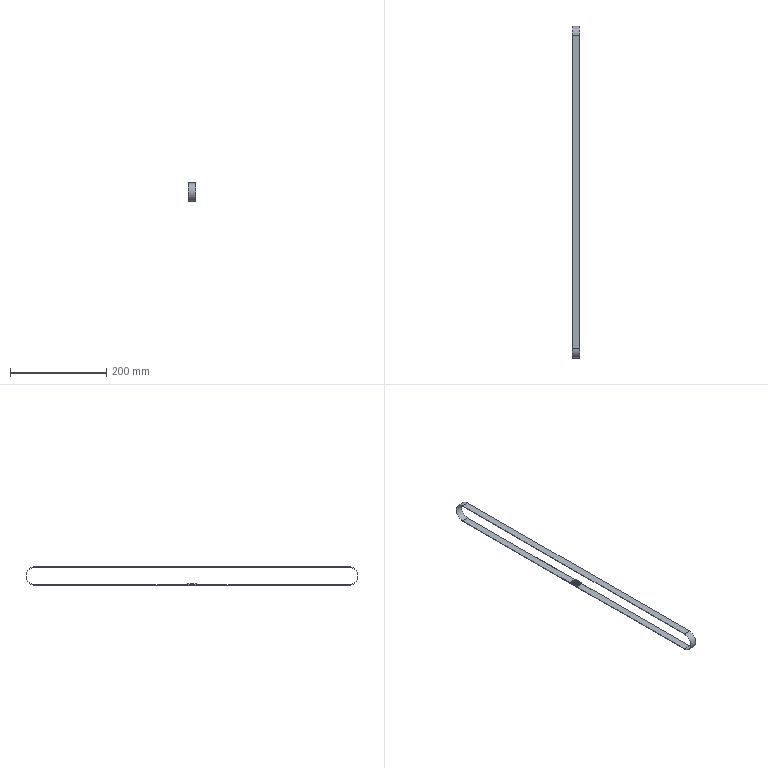Part | NX | features 5003_011_C-HTBN1350S5M-150 2 | 1 solid | 46 faces | box 15 x 688.836 x 38.84 mm | volume 17571 mm3 | plane 34 | cylinder 12 | commonest cylinder face diameters 6.5 x8 37.24 x2 38.84 x2
STEP:
#1=CARTESIAN_POINT('',(214.025,-206.042,-164.92));
#2=VERTEX_POINT('',#1);
#3=CARTESIAN_POINT('',(214.025,-206.877,-164.92));
#4=VERTEX_POINT('',#3);
#5=CARTESIAN_POINT('',(214.025,-205.127,-164.92));
#6=DIRECTION('',(0.,-1.,0.));
#7=VECTOR('',#6,1000.);
#8=LINE('',#5,#7);
#9=EDGE_CURVE('',#2,#4,#8,.T.);
#10=ORIENTED_EDGE('',*,*,#9,.F.);
#11=CARTESIAN_POINT('',(199.025,-206.042,-164.92));
#12=VERTEX_POINT('',#11);
#13=CARTESIAN_POINT('',(199.025,-206.042,-164.92));
#14=DIRECTION('',(1.,0.,0.));
#15=VECTOR('',#14,1000.);
#16=LINE('',#13,#15);
#17=EDGE_CURVE('',#12,#2,#16,.T.);
#18=ORIENTED_EDGE('',*,*,#17,.F.);
#19=CARTESIAN_POINT('',(199.025,-206.877,-164.92));
#20=VERTEX_POINT('',#19);
#21=CARTESIAN_POINT('',(199.025,-205.127,-164.92));
#22=DIRECTION('',(0.,-1.,0.));
#23=VECTOR('',#22,1000.);
#24=LINE('',#21,#23);
#25=EDGE_CURVE('',#12,#20,#24,.T.);
#26=ORIENTED_EDGE('',*,*,#25,.T.);
#27=CARTESIAN_POINT('',(214.025,-206.877,-164.92));
#28=DIRECTION('',(-1.,0.,0.));
#29=VECTOR('',#28,1000.);
#30=LINE('',#27,#29);
#31=EDGE_CURVE('',#4,#20,#30,.T.);
#32=ORIENTED_EDGE('',*,*,#31,.F.);
#33=EDGE_LOOP('',(#10,#18,#26,#32));
#34=FACE_BOUND('',#33,.T.);
#35=CARTESIAN_POINT('',(214.025,-205.127,-164.92));
#36=DIRECTION('',(0.,0.,-1.));
#37=DIRECTION('',(1.,0.,0.));
#38=AXIS2_PLACEMENT_3D('',#35,#36,#37);
#39=PLANE('',#38);
#40=ADVANCED_FACE('',(#34),#39,.F.);
#41=CARTESIAN_POINT('',(214.025,-201.042,-164.92));
#42=VERTEX_POINT('',#41);
#43=CARTESIAN_POINT('',(214.025,-201.877,-164.92));
#44=VERTEX_POINT('',#43);
#45=CARTESIAN_POINT('',(214.025,-201.002,-164.92));
#46=DIRECTION('',(0.,-1.,0.));
#47=VECTOR('',#46,1000.);
#48=LINE('',#45,#47);
#49=EDGE_CURVE('',#42,#44,#48,.T.);
#50=ORIENTED_EDGE('',*,*,#49,.F.);
#51=CARTESIAN_POINT('',(199.025,-201.042,-164.92));
#52=VERTEX_POINT('',#51);
#53=CARTESIAN_POINT('',(199.025,-201.042,-164.92));
#54=DIRECTION('',(1.,0.,0.));
#55=VECTOR('',#54,1000.);
#56=LINE('',#53,#55);
#57=EDGE_CURVE('',#52,#42,#56,.T.);
#58=ORIENTED_EDGE('',*,*,#57,.F.);
#59=CARTESIAN_POINT('',(199.025,-201.877,-164.92));
#60=VERTEX_POINT('',#59);
#61=CARTESIAN_POINT('',(199.025,-201.002,-164.92));
#62=DIRECTION('',(0.,-1.,0.));
#63=VECTOR('',#62,1000.);
#64=LINE('',#61,#63);
#65=EDGE_CURVE('',#52,#60,#64,.T.);
#66=ORIENTED_EDGE('',*,*,#65,.T.);
#67=CARTESIAN_POINT('',(214.025,-201.877,-164.92));
#68=DIRECTION('',(-1.,0.,0.));
#69=VECTOR('',#68,1000.);
#70=LINE('',#67,#69);
#71=EDGE_CURVE('',#44,#60,#70,.T.);
#72=ORIENTED_EDGE('',*,*,#71,.F.);
#73=EDGE_LOOP('',(#50,#58,#66,#72));
#74=FACE_BOUND('',#73,.T.);
#75=CARTESIAN_POINT('',(214.025,-201.002,-164.92));
#76=DIRECTION('',(0.,0.,-1.));
#77=DIRECTION('',(0.,1.,0.));
#78=AXIS2_PLACEMENT_3D('',#75,#76,#77);
#79=PLANE('',#78);
#80=ADVANCED_FACE('',(#74),#79,.F.);
#81=CARTESIAN_POINT('',(214.025,-196.042,-164.92));
#82=VERTEX_POINT('',#81);
#83=CARTESIAN_POINT('',(214.025,-196.877,-164.92));
#84=VERTEX_POINT('',#83);
#85=CARTESIAN_POINT('',(214.025,-195.127,-164.92));
#86=DIRECTION('',(0.,-1.,0.));
#87=VECTOR('',#86,1000.);
#88=LINE('',#85,#87);
#89=EDGE_CURVE('',#82,#84,#88,.T.);
#90=ORIENTED_EDGE('',*,*,#89,.F.);
#91=CARTESIAN_POINT('',(199.025,-196.042,-164.92));
#92=VERTEX_POINT('',#91);
#93=CARTESIAN_POINT('',(199.025,-196.042,-164.92));
#94=DIRECTION('',(1.,0.,0.));
#95=VECTOR('',#94,1000.);
#96=LINE('',#93,#95);
#97=EDGE_CURVE('',#92,#82,#96,.T.);
#98=ORIENTED_EDGE('',*,*,#97,.F.);
#99=CARTESIAN_POINT('',(199.025,-196.877,-164.92));
#100=VERTEX_POINT('',#99);
#101=CARTESIAN_POINT('',(199.025,-195.127,-164.92));
#102=DIRECTION('',(0.,-1.,0.));
#103=VECTOR('',#102,1000.);
#104=LINE('',#101,#103);
#105=EDGE_CURVE('',#92,#100,#104,.T.);
#106=ORIENTED_EDGE('',*,*,#105,.T.);
#107=CARTESIAN_POINT('',(214.025,-196.877,-164.92));
#108=DIRECTION('',(-1.,0.,0.));
#109=VECTOR('',#108,1000.);
#110=LINE('',#107,#109);
#111=EDGE_CURVE('',#84,#100,#110,.T.);
#112=ORIENTED_EDGE('',*,*,#111,.F.);
#113=EDGE_LOOP('',(#90,#98,#106,#112));
#114=FACE_BOUND('',#113,.T.);
#115=CARTESIAN_POINT('',(214.025,-195.127,-164.92));
#116=DIRECTION('',(0.,0.,-1.));
#117=DIRECTION('',(1.,0.,0.));
#118=AXIS2_PLACEMENT_3D('',#115,#116,#117);
#119=PLANE('',#118);
#120=ADVANCED_FACE('',(#114),#119,.F.);
#121=CARTESIAN_POINT('',(214.025,-526.,-165.62));
#122=VERTEX_POINT('',#121);
#123=CARTESIAN_POINT('',(214.025,-211.002,-165.62));
#124=VERTEX_POINT('',#123);
#125=CARTESIAN_POINT('',(214.025,123.996,-165.62));
#126=DIRECTION('',(0.,1.,0.));
#127=VECTOR('',#126,1000.);
#128=LINE('',#125,#127);
#129=EDGE_CURVE('',#122,#124,#128,.T.);
#130=ORIENTED_EDGE('',*,*,#129,.T.);
#131=CARTESIAN_POINT('',(199.025,-211.002,-165.62));
#132=VERTEX_POINT('',#131);
#133=CARTESIAN_POINT('',(214.025,-211.002,-165.62));
#134=DIRECTION('',(-1.,0.,0.));
#135=VECTOR('',#134,1000.);
#136=LINE('',#133,#135);
#137=EDGE_CURVE('',#124,#132,#136,.T.);
#138=ORIENTED_EDGE('',*,*,#137,.T.);
#139=CARTESIAN_POINT('',(199.025,-526.,-165.62));
#140=VERTEX_POINT('',#139);
#141=CARTESIAN_POINT('',(199.025,123.996,-165.62));
#142=DIRECTION('',(0.,1.,0.));
#143=VECTOR('',#142,1000.);
#144=LINE('',#141,#143);
#145=EDGE_CURVE('',#140,#132,#144,.T.);
#146=ORIENTED_EDGE('',*,*,#145,.F.);
#147=CARTESIAN_POINT('',(214.025,-526.,-165.62));
#148=DIRECTION('',(-1.,0.,0.));
#149=VECTOR('',#148,1000.);
#150=LINE('',#147,#149);
#151=EDGE_CURVE('',#122,#140,#150,.T.);
#152=ORIENTED_EDGE('',*,*,#151,.F.);
#153=EDGE_LOOP('',(#130,#138,#146,#152));
#154=FACE_BOUND('',#153,.T.);
#155=CARTESIAN_POINT('',(214.025,123.996,-165.62));
#156=DIRECTION('',(0.,0.,1.));
#157=DIRECTION('',(-1.,0.,0.));
#158=AXIS2_PLACEMENT_3D('',#155,#156,#157);
#159=PLANE('',#158);
#160=ADVANCED_FACE('',(#154),#159,.T.);
#161=CARTESIAN_POINT('',(199.025,-191.002,-165.62));
#162=VERTEX_POINT('',#161);
#163=CARTESIAN_POINT('',(199.025,123.996,-165.62));
#164=VERTEX_POINT('',#163);
#165=CARTESIAN_POINT('',(199.025,123.996,-165.62));
#166=DIRECTION('',(0.,1.,0.));
#167=VECTOR('',#166,1000.);
#168=LINE('',#165,#167);
#169=EDGE_CURVE('',#162,#164,#168,.T.);
#170=ORIENTED_EDGE('',*,*,#169,.F.);
#171=CARTESIAN_POINT('',(214.025,-191.002,-165.62));
#172=VERTEX_POINT('',#171);
#173=CARTESIAN_POINT('',(214.025,-191.002,-165.62));
#174=DIRECTION('',(1.,0.,0.));
#175=VECTOR('',#174,1000.);
#176=LINE('',#173,#175);
#177=EDGE_CURVE('',#162,#172,#176,.T.);
#178=ORIENTED_EDGE('',*,*,#177,.T.);
#179=CARTESIAN_POINT('',(214.025,123.996,-165.62));
#180=VERTEX_POINT('',#179);
#181=CARTESIAN_POINT('',(214.025,123.996,-165.62));
#182=DIRECTION('',(0.,1.,0.));
#183=VECTOR('',#182,1000.);
#184=LINE('',#181,#183);
#185=EDGE_CURVE('',#172,#180,#184,.T.);
#186=ORIENTED_EDGE('',*,*,#185,.T.);
#187=CARTESIAN_POINT('',(214.025,123.996,-165.62));
#188=DIRECTION('',(-1.,0.,0.));
#189=VECTOR('',#188,1000.);
#190=LINE('',#187,#189);
#191=EDGE_CURVE('',#180,#164,#190,.T.);
#192=ORIENTED_EDGE('',*,*,#191,.T.);
#193=EDGE_LOOP('',(#170,#178,#186,#192));
#194=FACE_BOUND('',#193,.T.);
#195=CARTESIAN_POINT('',(214.025,123.996,-165.62));
#196=DIRECTION('',(0.,0.,1.));
#197=DIRECTION('',(-1.,0.,0.));
#198=AXIS2_PLACEMENT_3D('',#195,#196,#197);
#199=PLANE('',#198);
#200=ADVANCED_FACE('',(#194),#199,.T.);
#201=CARTESIAN_POINT('',(214.025,-210.127,-164.92));
#202=VERTEX_POINT('',#201);
#203=CARTESIAN_POINT('',(214.025,-210.962,-164.92));
#204=VERTEX_POINT('',#203);
#205=CARTESIAN_POINT('',(214.025,-211.002,-164.92));
#206=DIRECTION('',(0.,-1.,0.));
#207=VECTOR('',#206,1000.);
#208=LINE('',#205,#207);
#209=EDGE_CURVE('',#202,#204,#208,.T.);
#210=ORIENTED_EDGE('',*,*,#209,.T.);
#211=CARTESIAN_POINT('',(214.025,-210.962,-164.96));
#212=VERTEX_POINT('',#211);
#213=CARTESIAN_POINT('',(214.025,-210.962,-164.92));
#214=DIRECTION('',(0.,0.,1.));
#215=VECTOR('',#214,1000.);
#216=LINE('',#213,#215);
#217=EDGE_CURVE('',#212,#204,#216,.T.);
#218=ORIENTED_EDGE('',*,*,#217,.F.);
#219=CARTESIAN_POINT('',(214.025,-211.002,-164.96));
#220=VERTEX_POINT('',#219);
#221=CARTESIAN_POINT('',(214.025,-210.962,-164.96));
#222=DIRECTION('',(0.,1.,0.));
#223=VECTOR('',#222,1000.);
#224=LINE('',#221,#223);
#225=EDGE_CURVE('',#220,#212,#224,.T.);
#226=ORIENTED_EDGE('',*,*,#225,.F.);
#227=CARTESIAN_POINT('',(214.025,-211.002,-166.42));
#228=DIRECTION('',(0.,0.,-1.));
#229=VECTOR('',#228,1000.);
#230=LINE('',#227,#229);
#231=EDGE_CURVE('',#220,#124,#230,.T.);
#232=ORIENTED_EDGE('',*,*,#231,.T.);
#233=ORIENTED_EDGE('',*,*,#129,.F.);
#234=CARTESIAN_POINT('',(214.025,-526.,-128.38));
#235=VERTEX_POINT('',#234);
#236=CARTESIAN_POINT('',(214.025,-526.,-147.));
#237=DIRECTION('',(1.,0.,0.));
#238=DIRECTION('',(0.,-1.,0.));
#239=AXIS2_PLACEMENT_3D('',#236,#237,#238);
#240=CIRCLE('',#239,18.62);
#241=EDGE_CURVE('',#235,#122,#240,.T.);
#242=ORIENTED_EDGE('',*,*,#241,.F.);
#243=CARTESIAN_POINT('',(214.025,123.996,-128.38));
#244=VERTEX_POINT('',#243);
#245=CARTESIAN_POINT('',(214.025,123.996,-128.38));
#246=DIRECTION('',(0.,-1.,0.));
#247=VECTOR('',#246,1000.);
#248=LINE('',#245,#247);
#249=EDGE_CURVE('',#244,#235,#248,.T.);
#250=ORIENTED_EDGE('',*,*,#249,.F.);
#251=CARTESIAN_POINT('',(214.025,123.996,-147.));
#252=DIRECTION('',(1.,0.,0.));
#253=DIRECTION('',(0.,-1.,0.));
#254=AXIS2_PLACEMENT_3D('',#251,#252,#253);
#255=CIRCLE('',#254,18.62);
#256=EDGE_CURVE('',#180,#244,#255,.T.);
#257=ORIENTED_EDGE('',*,*,#256,.F.);
#258=ORIENTED_EDGE('',*,*,#185,.F.);
#259=CARTESIAN_POINT('',(214.025,-191.002,-164.96));
#260=VERTEX_POINT('',#259);
#261=CARTESIAN_POINT('',(214.025,-191.002,-164.92));
#262=DIRECTION('',(0.,0.,1.));
#263=VECTOR('',#262,1000.);
#264=LINE('',#261,#263);
#265=EDGE_CURVE('',#172,#260,#264,.T.);
#266=ORIENTED_EDGE('',*,*,#265,.T.);
#267=CARTESIAN_POINT('',(214.025,-191.042,-164.96));
#268=VERTEX_POINT('',#267);
#269=CARTESIAN_POINT('',(214.025,-190.962,-164.96));
#270=DIRECTION('',(0.,1.,0.));
#271=VECTOR('',#270,1000.);
#272=LINE('',#269,#271);
#273=EDGE_CURVE('',#268,#260,#272,.T.);
#274=ORIENTED_EDGE('',*,*,#273,.F.);
#275=CARTESIAN_POINT('',(214.025,-191.042,-164.92));
#276=VERTEX_POINT('',#275);
#277=CARTESIAN_POINT('',(214.025,-191.042,-164.96));
#278=DIRECTION('',(0.,0.,-1.));
#279=VECTOR('',#278,1000.);
#280=LINE('',#277,#279);
#281=EDGE_CURVE('',#276,#268,#280,.T.);
#282=ORIENTED_EDGE('',*,*,#281,.F.);
#283=CARTESIAN_POINT('',(214.025,-191.877,-164.92));
#284=VERTEX_POINT('',#283);
#285=CARTESIAN_POINT('',(214.025,-191.877,-164.92));
#286=DIRECTION('',(0.,-1.,0.));
#287=VECTOR('',#286,1000.);
#288=LINE('',#285,#287);
#289=EDGE_CURVE('',#276,#284,#288,.T.);
#290=ORIENTED_EDGE('',*,*,#289,.T.);
#291=CARTESIAN_POINT('',(214.025,-192.498,-163.01));
#292=VERTEX_POINT('',#291);
#293=CARTESIAN_POINT('',(214.025,-195.127,-164.92));
#294=DIRECTION('',(1.,0.,0.));
#295=DIRECTION('',(0.,-1.,0.));
#296=AXIS2_PLACEMENT_3D('',#293,#294,#295);
#297=CIRCLE('',#296,3.25);
#298=EDGE_CURVE('',#284,#292,#297,.T.);
#299=ORIENTED_EDGE('',*,*,#298,.T.);
#300=CARTESIAN_POINT('',(214.025,-194.507,-163.01));
#301=VERTEX_POINT('',#300);
#302=CARTESIAN_POINT('',(214.025,-192.498,-163.01));
#303=DIRECTION('',(0.,-1.,0.));
#304=VECTOR('',#303,1000.);
#305=LINE('',#302,#304);
#306=EDGE_CURVE('',#292,#301,#305,.T.);
#307=ORIENTED_EDGE('',*,*,#306,.T.);
#308=CARTESIAN_POINT('',(214.025,-195.127,-164.92));
#309=VERTEX_POINT('',#308);
#310=CARTESIAN_POINT('',(214.025,-191.877,-164.92));
#311=DIRECTION('',(1.,0.,0.));
#312=DIRECTION('',(0.,-1.,0.));
#313=AXIS2_PLACEMENT_3D('',#310,#311,#312);
#314=CIRCLE('',#313,3.25);
#315=EDGE_CURVE('',#301,#309,#314,.T.);
#316=ORIENTED_EDGE('',*,*,#315,.T.);
#317=CARTESIAN_POINT('',(214.025,-195.962,-164.92));
#318=VERTEX_POINT('',#317);
#319=CARTESIAN_POINT('',(214.025,-195.127,-164.92));
#320=DIRECTION('',(0.,-1.,0.));
#321=VECTOR('',#320,1000.);
#322=LINE('',#319,#321);
#323=EDGE_CURVE('',#309,#318,#322,.T.);
#324=ORIENTED_EDGE('',*,*,#323,.T.);
#325=CARTESIAN_POINT('',(214.025,-195.962,-164.96));
#326=VERTEX_POINT('',#325);
#327=CARTESIAN_POINT('',(214.025,-195.962,-164.92));
#328=DIRECTION('',(0.,0.,1.));
#329=VECTOR('',#328,1000.);
#330=LINE('',#327,#329);
#331=EDGE_CURVE('',#326,#318,#330,.T.);
#332=ORIENTED_EDGE('',*,*,#331,.F.);
#333=CARTESIAN_POINT('',(214.025,-196.042,-164.96));
#334=VERTEX_POINT('',#333);
#335=CARTESIAN_POINT('',(214.025,-195.962,-164.96));
#336=DIRECTION('',(0.,1.,0.));
#337=VECTOR('',#336,1000.);
#338=LINE('',#335,#337);
#339=EDGE_CURVE('',#334,#326,#338,.T.);
#340=ORIENTED_EDGE('',*,*,#339,.F.);
#341=CARTESIAN_POINT('',(214.025,-196.042,-164.96));
#342=DIRECTION('',(0.,0.,-1.));
#343=VECTOR('',#342,1000.);
#344=LINE('',#341,#343);
#345=EDGE_CURVE('',#82,#334,#344,.T.);
#346=ORIENTED_EDGE('',*,*,#345,.F.);
#347=ORIENTED_EDGE('',*,*,#89,.T.);
#348=CARTESIAN_POINT('',(214.025,-197.498,-163.01));
#349=VERTEX_POINT('',#348);
#350=CARTESIAN_POINT('',(214.025,-200.127,-164.92));
#351=DIRECTION('',(1.,0.,0.));
#352=DIRECTION('',(0.,-1.,0.));
#353=AXIS2_PLACEMENT_3D('',#350,#351,#352);
#354=CIRCLE('',#353,3.25);
#355=EDGE_CURVE('',#84,#349,#354,.T.);
#356=ORIENTED_EDGE('',*,*,#355,.T.);
#357=CARTESIAN_POINT('',(214.025,-199.507,-163.01));
#358=VERTEX_POINT('',#357);
#359=CARTESIAN_POINT('',(214.025,-197.498,-163.01));
#360=DIRECTION('',(0.,-1.,0.));
#361=VECTOR('',#360,1000.);
#362=LINE('',#359,#361);
#363=EDGE_CURVE('',#349,#358,#362,.T.);
#364=ORIENTED_EDGE('',*,*,#363,.T.);
#365=CARTESIAN_POINT('',(214.025,-200.127,-164.92));
#366=VERTEX_POINT('',#365);
#367=CARTESIAN_POINT('',(214.025,-196.877,-164.92));
#368=DIRECTION('',(1.,0.,0.));
#369=DIRECTION('',(0.,-1.,0.));
#370=AXIS2_PLACEMENT_3D('',#367,#368,#369);
#371=CIRCLE('',#370,3.25);
#372=EDGE_CURVE('',#358,#366,#371,.T.);
#373=ORIENTED_EDGE('',*,*,#372,.T.);
#374=CARTESIAN_POINT('',(214.025,-200.962,-164.92));
#375=VERTEX_POINT('',#374);
#376=CARTESIAN_POINT('',(214.025,-201.002,-164.92));
#377=DIRECTION('',(0.,-1.,0.));
#378=VECTOR('',#377,1000.);
#379=LINE('',#376,#378);
#380=EDGE_CURVE('',#366,#375,#379,.T.);
#381=ORIENTED_EDGE('',*,*,#380,.T.);
#382=CARTESIAN_POINT('',(214.025,-200.962,-164.96));
#383=VERTEX_POINT('',#382);
#384=CARTESIAN_POINT('',(214.025,-200.962,-164.92));
#385=DIRECTION('',(0.,0.,1.));
#386=VECTOR('',#385,1000.);
#387=LINE('',#384,#386);
#388=EDGE_CURVE('',#383,#375,#387,.T.);
#389=ORIENTED_EDGE('',*,*,#388,.F.);
#390=CARTESIAN_POINT('',(214.025,-201.042,-164.96));
#391=VERTEX_POINT('',#390);
#392=CARTESIAN_POINT('',(214.025,-200.962,-164.96));
#393=DIRECTION('',(0.,1.,0.));
#394=VECTOR('',#393,1000.);
#395=LINE('',#392,#394);
#396=EDGE_CURVE('',#391,#383,#395,.T.);
#397=ORIENTED_EDGE('',*,*,#396,.F.);
#398=CARTESIAN_POINT('',(214.025,-201.042,-164.96));
#399=DIRECTION('',(0.,0.,-1.));
#400=VECTOR('',#399,1000.);
#401=LINE('',#398,#400);
#402=EDGE_CURVE('',#42,#391,#401,.T.);
#403=ORIENTED_EDGE('',*,*,#402,.F.);
#404=ORIENTED_EDGE('',*,*,#49,.T.);
#405=CARTESIAN_POINT('',(214.025,-202.498,-163.01));
#406=VERTEX_POINT('',#405);
#407=CARTESIAN_POINT('',(214.025,-205.127,-164.92));
#408=DIRECTION('',(1.,0.,0.));
#409=DIRECTION('',(0.,-1.,0.));
#410=AXIS2_PLACEMENT_3D('',#407,#408,#409);
#411=CIRCLE('',#410,3.25);
#412=EDGE_CURVE('',#44,#406,#411,.T.);
#413=ORIENTED_EDGE('',*,*,#412,.T.);
#414=CARTESIAN_POINT('',(214.025,-204.507,-163.01));
#415=VERTEX_POINT('',#414);
#416=CARTESIAN_POINT('',(214.025,-202.498,-163.01));
#417=DIRECTION('',(0.,-1.,0.));
#418=VECTOR('',#417,1000.);
#419=LINE('',#416,#418);
#420=EDGE_CURVE('',#406,#415,#419,.T.);
#421=ORIENTED_EDGE('',*,*,#420,.T.);
#422=CARTESIAN_POINT('',(214.025,-205.127,-164.92));
#423=VERTEX_POINT('',#422);
#424=CARTESIAN_POINT('',(214.025,-201.877,-164.92));
#425=DIRECTION('',(1.,0.,0.));
#426=DIRECTION('',(0.,-1.,0.));
#427=AXIS2_PLACEMENT_3D('',#424,#425,#426);
#428=CIRCLE('',#427,3.25);
#429=EDGE_CURVE('',#415,#423,#428,.T.);
#430=ORIENTED_EDGE('',*,*,#429,.T.);
#431=CARTESIAN_POINT('',(214.025,-205.962,-164.92));
#432=VERTEX_POINT('',#431);
#433=CARTESIAN_POINT('',(214.025,-205.127,-164.92));
#434=DIRECTION('',(0.,-1.,0.));
#435=VECTOR('',#434,1000.);
#436=LINE('',#433,#435);
#437=EDGE_CURVE('',#423,#432,#436,.T.);
#438=ORIENTED_EDGE('',*,*,#437,.T.);
#439=CARTESIAN_POINT('',(214.025,-205.962,-164.96));
#440=VERTEX_POINT('',#439);
#441=CARTESIAN_POINT('',(214.025,-205.962,-164.92));
#442=DIRECTION('',(0.,0.,1.));
#443=VECTOR('',#442,1000.);
#444=LINE('',#441,#443);
#445=EDGE_CURVE('',#440,#432,#444,.T.);
#446=ORIENTED_EDGE('',*,*,#445,.F.);
#447=CARTESIAN_POINT('',(214.025,-206.042,-164.96));
#448=VERTEX_POINT('',#447);
#449=CARTESIAN_POINT('',(214.025,-205.962,-164.96));
#450=DIRECTION('',(0.,1.,0.));
#451=VECTOR('',#450,1000.);
#452=LINE('',#449,#451);
#453=EDGE_CURVE('',#448,#440,#452,.T.);
#454=ORIENTED_EDGE('',*,*,#453,.F.);
#455=CARTESIAN_POINT('',(214.025,-206.042,-164.96));
#456=DIRECTION('',(0.,0.,-1.));
#457=VECTOR('',#456,1000.);
#458=LINE('',#455,#457);
#459=EDGE_CURVE('',#2,#448,#458,.T.);
#460=ORIENTED_EDGE('',*,*,#459,.F.);
#461=ORIENTED_EDGE('',*,*,#9,.T.);
#462=CARTESIAN_POINT('',(214.025,-207.498,-163.01));
#463=VERTEX_POINT('',#462);
#464=CARTESIAN_POINT('',(214.025,-210.127,-164.92));
#465=DIRECTION('',(1.,0.,0.));
#466=DIRECTION('',(0.,-1.,0.));
#467=AXIS2_PLACEMENT_3D('',#464,#465,#466);
#468=CIRCLE('',#467,3.25);
#469=EDGE_CURVE('',#4,#463,#468,.T.);
#470=ORIENTED_EDGE('',*,*,#469,.T.);
#471=CARTESIAN_POINT('',(214.025,-209.507,-163.01));
#472=VERTEX_POINT('',#471);
#473=CARTESIAN_POINT('',(214.025,-207.498,-163.01));
#474=DIRECTION('',(0.,-1.,0.));
#475=VECTOR('',#474,1000.);
#476=LINE('',#473,#475);
#477=EDGE_CURVE('',#463,#472,#476,.T.);
#478=ORIENTED_EDGE('',*,*,#477,.T.);
#479=CARTESIAN_POINT('',(214.025,-206.877,-164.92));
#480=DIRECTION('',(1.,0.,0.));
#481=DIRECTION('',(0.,-1.,0.));
#482=AXIS2_PLACEMENT_3D('',#479,#480,#481);
#483=CIRCLE('',#482,3.25);
#484=EDGE_CURVE('',#472,#202,#483,.T.);
#485=ORIENTED_EDGE('',*,*,#484,.T.);
#486=EDGE_LOOP('',(#210,#218,#226,#232,#233,#242,#250,#257,#258,#266,#274,#282,#290,#299,#307,#316,#324,#332,#340,#346,#347,#356,#364,#373,#381,#389,#397,#403,#404,#413,#421,#430,#438,#446,#454,#460,#461,#470,#478,#485));
#487=FACE_BOUND('',#486,.T.);
#488=CARTESIAN_POINT('',(214.025,-526.,-166.42));
#489=VERTEX_POINT('',#488);
#490=CARTESIAN_POINT('',(214.025,123.996,-166.42));
#491=VERTEX_POINT('',#490);
#492=CARTESIAN_POINT('',(214.025,123.996,-166.42));
#493=DIRECTION('',(0.,1.,0.));
#494=VECTOR('',#493,1000.);
#495=LINE('',#492,#494);
#496=EDGE_CURVE('',#489,#491,#495,.T.);
#497=ORIENTED_EDGE('',*,*,#496,.T.);
#498=CARTESIAN_POINT('',(214.025,123.996,-127.58));
#499=VERTEX_POINT('',#498);
#500=CARTESIAN_POINT('',(214.025,123.996,-147.));
#501=DIRECTION('',(1.,0.,0.));
#502=DIRECTION('',(0.,1.,0.));
#503=AXIS2_PLACEMENT_3D('',#500,#501,#502);
#504=CIRCLE('',#503,19.42);
#505=EDGE_CURVE('',#491,#499,#504,.T.);
#506=ORIENTED_EDGE('',*,*,#505,.T.);
#507=CARTESIAN_POINT('',(214.025,-526.,-127.58));
#508=VERTEX_POINT('',#507);
#509=CARTESIAN_POINT('',(214.025,123.996,-127.58));
#510=DIRECTION('',(0.,-1.,0.));
#511=VECTOR('',#510,1000.);
#512=LINE('',#509,#511);
#513=EDGE_CURVE('',#499,#508,#512,.T.);
#514=ORIENTED_EDGE('',*,*,#513,.T.);
#515=CARTESIAN_POINT('',(214.025,-526.,-147.));
#516=DIRECTION('',(1.,0.,0.));
#517=DIRECTION('',(0.,1.,0.));
#518=AXIS2_PLACEMENT_3D('',#515,#516,#517);
#519=CIRCLE('',#518,19.42);
#520=EDGE_CURVE('',#508,#489,#519,.T.);
#521=ORIENTED_EDGE('',*,*,#520,.T.);
#522=EDGE_LOOP('',(#497,#506,#514,#521));
#523=FACE_BOUND('',#522,.T.);
#524=CARTESIAN_POINT('',(214.025,123.996,-147.));
#525=DIRECTION('',(-1.,0.,0.));
#526=DIRECTION('',(0.,1.,0.));
#527=AXIS2_PLACEMENT_3D('',#524,#525,#526);
#528=PLANE('',#527);
#529=ADVANCED_FACE('',(#487,#523),#528,.F.);
#530=CARTESIAN_POINT('',(199.025,-210.962,-164.96));
#531=VERTEX_POINT('',#530);
#532=CARTESIAN_POINT('',(199.025,-210.962,-164.92));
#533=VERTEX_POINT('',#532);
#534=CARTESIAN_POINT('',(199.025,-210.962,-164.92));
#535=DIRECTION('',(0.,0.,1.));
#536=VECTOR('',#535,1000.);
#537=LINE('',#534,#536);
#538=EDGE_CURVE('',#531,#533,#537,.T.);
#539=ORIENTED_EDGE('',*,*,#538,.T.);
#540=CARTESIAN_POINT('',(199.025,-210.127,-164.92));
#541=VERTEX_POINT('',#540);
#542=CARTESIAN_POINT('',(199.025,-211.002,-164.92));
#543=DIRECTION('',(0.,-1.,0.));
#544=VECTOR('',#543,1000.);
#545=LINE('',#542,#544);
#546=EDGE_CURVE('',#541,#533,#545,.T.);
#547=ORIENTED_EDGE('',*,*,#546,.F.);
#548=CARTESIAN_POINT('',(199.025,-209.507,-163.01));
#549=VERTEX_POINT('',#548);
#550=CARTESIAN_POINT('',(199.025,-206.877,-164.92));
#551=DIRECTION('',(1.,0.,0.));
#552=DIRECTION('',(0.,-1.,0.));
#553=AXIS2_PLACEMENT_3D('',#550,#551,#552);
#554=CIRCLE('',#553,3.25);
#555=EDGE_CURVE('',#549,#541,#554,.T.);
#556=ORIENTED_EDGE('',*,*,#555,.F.);
#557=CARTESIAN_POINT('',(199.025,-207.498,-163.01));
#558=VERTEX_POINT('',#557);
#559=CARTESIAN_POINT('',(199.025,-207.498,-163.01));
#560=DIRECTION('',(0.,-1.,0.));
#561=VECTOR('',#560,1000.);
#562=LINE('',#559,#561);
#563=EDGE_CURVE('',#558,#549,#562,.T.);
#564=ORIENTED_EDGE('',*,*,#563,.F.);
#565=CARTESIAN_POINT('',(199.025,-210.127,-164.92));
#566=DIRECTION('',(1.,0.,0.));
#567=DIRECTION('',(0.,-1.,0.));
#568=AXIS2_PLACEMENT_3D('',#565,#566,#567);
#569=CIRCLE('',#568,3.25);
#570=EDGE_CURVE('',#20,#558,#569,.T.);
#571=ORIENTED_EDGE('',*,*,#570,.F.);
#572=ORIENTED_EDGE('',*,*,#25,.F.);
#573=CARTESIAN_POINT('',(199.025,-206.042,-164.96));
#574=VERTEX_POINT('',#573);
#575=CARTESIAN_POINT('',(199.025,-206.042,-164.96));
#576=DIRECTION('',(0.,0.,-1.));
#577=VECTOR('',#576,1000.);
#578=LINE('',#575,#577);
#579=EDGE_CURVE('',#12,#574,#578,.T.);
#580=ORIENTED_EDGE('',*,*,#579,.T.);
#581=CARTESIAN_POINT('',(199.025,-205.962,-164.96));
#582=VERTEX_POINT('',#581);
#583=CARTESIAN_POINT('',(199.025,-205.962,-164.96));
#584=DIRECTION('',(0.,1.,0.));
#585=VECTOR('',#584,1000.);
#586=LINE('',#583,#585);
#587=EDGE_CURVE('',#574,#582,#586,.T.);
#588=ORIENTED_EDGE('',*,*,#587,.T.);
#589=CARTESIAN_POINT('',(199.025,-205.962,-164.92));
#590=VERTEX_POINT('',#589);
#591=CARTESIAN_POINT('',(199.025,-205.962,-164.92));
#592=DIRECTION('',(0.,0.,1.));
#593=VECTOR('',#592,1000.);
#594=LINE('',#591,#593);
#595=EDGE_CURVE('',#582,#590,#594,.T.);
#596=ORIENTED_EDGE('',*,*,#595,.T.);
#597=CARTESIAN_POINT('',(199.025,-205.127,-164.92));
#598=VERTEX_POINT('',#597);
#599=CARTESIAN_POINT('',(199.025,-205.127,-164.92));
#600=DIRECTION('',(0.,-1.,0.));
#601=VECTOR('',#600,1000.);
#602=LINE('',#599,#601);
#603=EDGE_CURVE('',#598,#590,#602,.T.);
#604=ORIENTED_EDGE('',*,*,#603,.F.);
#605=CARTESIAN_POINT('',(199.025,-204.507,-163.01));
#606=VERTEX_POINT('',#605);
#607=CARTESIAN_POINT('',(199.025,-201.877,-164.92));
#608=DIRECTION('',(1.,0.,0.));
#609=DIRECTION('',(0.,-1.,0.));
#610=AXIS2_PLACEMENT_3D('',#607,#608,#609);
#611=CIRCLE('',#610,3.25);
#612=EDGE_CURVE('',#606,#598,#611,.T.);
#613=ORIENTED_EDGE('',*,*,#612,.F.);
#614=CARTESIAN_POINT('',(199.025,-202.498,-163.01));
#615=VERTEX_POINT('',#614);
#616=CARTESIAN_POINT('',(199.025,-202.498,-163.01));
#617=DIRECTION('',(0.,-1.,0.));
#618=VECTOR('',#617,1000.);
#619=LINE('',#616,#618);
#620=EDGE_CURVE('',#615,#606,#619,.T.);
#621=ORIENTED_EDGE('',*,*,#620,.F.);
#622=CARTESIAN_POINT('',(199.025,-205.127,-164.92));
#623=DIRECTION('',(1.,0.,0.));
#624=DIRECTION('',(0.,-1.,0.));
#625=AXIS2_PLACEMENT_3D('',#622,#623,#624);
#626=CIRCLE('',#625,3.25);
#627=EDGE_CURVE('',#60,#615,#626,.T.);
#628=ORIENTED_EDGE('',*,*,#627,.F.);
#629=ORIENTED_EDGE('',*,*,#65,.F.);
#630=CARTESIAN_POINT('',(199.025,-201.042,-164.96));
#631=VERTEX_POINT('',#630);
#632=CARTESIAN_POINT('',(199.025,-201.042,-164.96));
#633=DIRECTION('',(0.,0.,-1.));
#634=VECTOR('',#633,1000.);
#635=LINE('',#632,#634);
#636=EDGE_CURVE('',#52,#631,#635,.T.);
#637=ORIENTED_EDGE('',*,*,#636,.T.);
#638=CARTESIAN_POINT('',(199.025,-200.962,-164.96));
#639=VERTEX_POINT('',#638);
#640=CARTESIAN_POINT('',(199.025,-200.962,-164.96));
#641=DIRECTION('',(0.,1.,0.));
#642=VECTOR('',#641,1000.);
#643=LINE('',#640,#642);
#644=EDGE_CURVE('',#631,#639,#643,.T.);
#645=ORIENTED_EDGE('',*,*,#644,.T.);
#646=CARTESIAN_POINT('',(199.025,-200.962,-164.92));
#647=VERTEX_POINT('',#646);
#648=CARTESIAN_POINT('',(199.025,-200.962,-164.92));
#649=DIRECTION('',(0.,0.,1.));
#650=VECTOR('',#649,1000.);
#651=LINE('',#648,#650);
#652=EDGE_CURVE('',#639,#647,#651,.T.);
#653=ORIENTED_EDGE('',*,*,#652,.T.);
#654=CARTESIAN_POINT('',(199.025,-200.127,-164.92));
#655=VERTEX_POINT('',#654);
#656=CARTESIAN_POINT('',(199.025,-201.002,-164.92));
#657=DIRECTION('',(0.,-1.,0.));
#658=VECTOR('',#657,1000.);
#659=LINE('',#656,#658);
#660=EDGE_CURVE('',#655,#647,#659,.T.);
#661=ORIENTED_EDGE('',*,*,#660,.F.);
#662=CARTESIAN_POINT('',(199.025,-199.507,-163.01));
#663=VERTEX_POINT('',#662);
#664=CARTESIAN_POINT('',(199.025,-196.877,-164.92));
#665=DIRECTION('',(1.,0.,0.));
#666=DIRECTION('',(0.,-1.,0.));
#667=AXIS2_PLACEMENT_3D('',#664,#665,#666);
#668=CIRCLE('',#667,3.25);
#669=EDGE_CURVE('',#663,#655,#668,.T.);
#670=ORIENTED_EDGE('',*,*,#669,.F.);
#671=CARTESIAN_POINT('',(199.025,-197.498,-163.01));
#672=VERTEX_POINT('',#671);
#673=CARTESIAN_POINT('',(199.025,-197.498,-163.01));
#674=DIRECTION('',(0.,-1.,0.));
#675=VECTOR('',#674,1000.);
#676=LINE('',#673,#675);
#677=EDGE_CURVE('',#672,#663,#676,.T.);
#678=ORIENTED_EDGE('',*,*,#677,.F.);
#679=CARTESIAN_POINT('',(199.025,-200.127,-164.92));
#680=DIRECTION('',(1.,0.,0.));
#681=DIRECTION('',(0.,-1.,0.));
#682=AXIS2_PLACEMENT_3D('',#679,#680,#681);
#683=CIRCLE('',#682,3.25);
#684=EDGE_CURVE('',#100,#672,#683,.T.);
#685=ORIENTED_EDGE('',*,*,#684,.F.);
#686=ORIENTED_EDGE('',*,*,#105,.F.);
#687=CARTESIAN_POINT('',(199.025,-196.042,-164.96));
#688=VERTEX_POINT('',#687);
#689=CARTESIAN_POINT('',(199.025,-196.042,-164.96));
#690=DIRECTION('',(0.,0.,-1.));
#691=VECTOR('',#690,1000.);
#692=LINE('',#689,#691);
#693=EDGE_CURVE('',#92,#688,#692,.T.);
#694=ORIENTED_EDGE('',*,*,#693,.T.);
#695=CARTESIAN_POINT('',(199.025,-195.962,-164.96));
#696=VERTEX_POINT('',#695);
#697=CARTESIAN_POINT('',(199.025,-195.962,-164.96));
#698=DIRECTION('',(0.,1.,0.));
#699=VECTOR('',#698,1000.);
#700=LINE('',#697,#699);
#701=EDGE_CURVE('',#688,#696,#700,.T.);
#702=ORIENTED_EDGE('',*,*,#701,.T.);
#703=CARTESIAN_POINT('',(199.025,-195.962,-164.92));
#704=VERTEX_POINT('',#703);
#705=CARTESIAN_POINT('',(199.025,-195.962,-164.92));
#706=DIRECTION('',(0.,0.,1.));
#707=VECTOR('',#706,1000.);
#708=LINE('',#705,#707);
#709=EDGE_CURVE('',#696,#704,#708,.T.);
#710=ORIENTED_EDGE('',*,*,#709,.T.);
#711=CARTESIAN_POINT('',(199.025,-195.127,-164.92));
#712=VERTEX_POINT('',#711);
#713=CARTESIAN_POINT('',(199.025,-195.127,-164.92));
#714=DIRECTION('',(0.,-1.,0.));
#715=VECTOR('',#714,1000.);
#716=LINE('',#713,#715);
#717=EDGE_CURVE('',#712,#704,#716,.T.);
#718=ORIENTED_EDGE('',*,*,#717,.F.);
#719=CARTESIAN_POINT('',(199.025,-194.507,-163.01));
#720=VERTEX_POINT('',#719);
#721=CARTESIAN_POINT('',(199.025,-191.877,-164.92));
#722=DIRECTION('',(1.,0.,0.));
#723=DIRECTION('',(0.,-1.,0.));
#724=AXIS2_PLACEMENT_3D('',#721,#722,#723);
#725=CIRCLE('',#724,3.25);
#726=EDGE_CURVE('',#720,#712,#725,.T.);
#727=ORIENTED_EDGE('',*,*,#726,.F.);
#728=CARTESIAN_POINT('',(199.025,-192.498,-163.01));
#729=VERTEX_POINT('',#728);
#730=CARTESIAN_POINT('',(199.025,-192.498,-163.01));
#731=DIRECTION('',(0.,-1.,0.));
#732=VECTOR('',#731,1000.);
#733=LINE('',#730,#732);
#734=EDGE_CURVE('',#729,#720,#733,.T.);
#735=ORIENTED_EDGE('',*,*,#734,.F.);
#736=CARTESIAN_POINT('',(199.025,-191.877,-164.92));
#737=VERTEX_POINT('',#736);
#738=CARTESIAN_POINT('',(199.025,-195.127,-164.92));
#739=DIRECTION('',(1.,0.,0.));
#740=DIRECTION('',(0.,-1.,0.));
#741=AXIS2_PLACEMENT_3D('',#738,#739,#740);
#742=CIRCLE('',#741,3.25);
#743=EDGE_CURVE('',#737,#729,#742,.T.);
#744=ORIENTED_EDGE('',*,*,#743,.F.);
#745=CARTESIAN_POINT('',(199.025,-191.042,-164.92));
#746=VERTEX_POINT('',#745);
#747=CARTESIAN_POINT('',(199.025,-191.877,-164.92));
#748=DIRECTION('',(0.,-1.,0.));
#749=VECTOR('',#748,1000.);
#750=LINE('',#747,#749);
#751=EDGE_CURVE('',#746,#737,#750,.T.);
#752=ORIENTED_EDGE('',*,*,#751,.F.);
#753=CARTESIAN_POINT('',(199.025,-191.042,-164.96));
#754=VERTEX_POINT('',#753);
#755=CARTESIAN_POINT('',(199.025,-191.042,-164.96));
#756=DIRECTION('',(0.,0.,-1.));
#757=VECTOR('',#756,1000.);
#758=LINE('',#755,#757);
#759=EDGE_CURVE('',#746,#754,#758,.T.);
#760=ORIENTED_EDGE('',*,*,#759,.T.);
#761=CARTESIAN_POINT('',(199.025,-191.002,-164.96));
#762=VERTEX_POINT('',#761);
#763=CARTESIAN_POINT('',(199.025,-190.962,-164.96));
#764=DIRECTION('',(0.,1.,0.));
#765=VECTOR('',#764,1000.);
#766=LINE('',#763,#765);
#767=EDGE_CURVE('',#754,#762,#766,.T.);
#768=ORIENTED_EDGE('',*,*,#767,.T.);
#769=CARTESIAN_POINT('',(199.025,-191.002,-164.92));
#770=DIRECTION('',(0.,0.,1.));
#771=VECTOR('',#770,1000.);
#772=LINE('',#769,#771);
#773=EDGE_CURVE('',#162,#762,#772,.T.);
#774=ORIENTED_EDGE('',*,*,#773,.F.);
#775=ORIENTED_EDGE('',*,*,#169,.T.);
#776=CARTESIAN_POINT('',(199.025,123.996,-128.38));
#777=VERTEX_POINT('',#776);
#778=CARTESIAN_POINT('',(199.025,123.996,-147.));
#779=DIRECTION('',(1.,0.,0.));
#780=DIRECTION('',(0.,-1.,0.));
#781=AXIS2_PLACEMENT_3D('',#778,#779,#780);
#782=CIRCLE('',#781,18.62);
#783=EDGE_CURVE('',#164,#777,#782,.T.);
#784=ORIENTED_EDGE('',*,*,#783,.T.);
#785=CARTESIAN_POINT('',(199.025,-526.,-128.38));
#786=VERTEX_POINT('',#785);
#787=CARTESIAN_POINT('',(199.025,123.996,-128.38));
#788=DIRECTION('',(0.,-1.,0.));
#789=VECTOR('',#788,1000.);
#790=LINE('',#787,#789);
#791=EDGE_CURVE('',#777,#786,#790,.T.);
#792=ORIENTED_EDGE('',*,*,#791,.T.);
#793=CARTESIAN_POINT('',(199.025,-526.,-147.));
#794=DIRECTION('',(1.,0.,0.));
#795=DIRECTION('',(0.,-1.,0.));
#796=AXIS2_PLACEMENT_3D('',#793,#794,#795);
#797=CIRCLE('',#796,18.62);
#798=EDGE_CURVE('',#786,#140,#797,.T.);
#799=ORIENTED_EDGE('',*,*,#798,.T.);
#800=ORIENTED_EDGE('',*,*,#145,.T.);
#801=CARTESIAN_POINT('',(199.025,-211.002,-164.96));
#802=VERTEX_POINT('',#801);
#803=CARTESIAN_POINT('',(199.025,-211.002,-166.42));
#804=DIRECTION('',(0.,0.,-1.));
#805=VECTOR('',#804,1000.);
#806=LINE('',#803,#805);
#807=EDGE_CURVE('',#802,#132,#806,.T.);
#808=ORIENTED_EDGE('',*,*,#807,.F.);
#809=CARTESIAN_POINT('',(199.025,-210.962,-164.96));
#810=DIRECTION('',(0.,1.,0.));
#811=VECTOR('',#810,1000.);
#812=LINE('',#809,#811);
#813=EDGE_CURVE('',#802,#531,#812,.T.);
#814=ORIENTED_EDGE('',*,*,#813,.T.);
#815=EDGE_LOOP('',(#539,#547,#556,#564,#571,#572,#580,#588,#596,#604,#613,#621,#628,#629,#637,#645,#653,#661,#670,#678,#685,#686,#694,#702,#710,#718,#727,#735,#744,#752,#760,#768,#774,#775,#784,#792,#799,#800,#808,#814));
#816=FACE_BOUND('',#815,.T.);
#817=CARTESIAN_POINT('',(199.025,123.996,-166.42));
#818=VERTEX_POINT('',#817);
#819=CARTESIAN_POINT('',(199.025,123.996,-127.58));
#820=VERTEX_POINT('',#819);
#821=CARTESIAN_POINT('',(199.025,123.996,-147.));
#822=DIRECTION('',(1.,0.,0.));
#823=DIRECTION('',(0.,1.,0.));
#824=AXIS2_PLACEMENT_3D('',#821,#822,#823);
#825=CIRCLE('',#824,19.42);
#826=EDGE_CURVE('',#818,#820,#825,.T.);
#827=ORIENTED_EDGE('',*,*,#826,.F.);
#828=CARTESIAN_POINT('',(199.025,-526.,-166.42));
#829=VERTEX_POINT('',#828);
#830=CARTESIAN_POINT('',(199.025,123.996,-166.42));
#831=DIRECTION('',(0.,1.,0.));
#832=VECTOR('',#831,1000.);
#833=LINE('',#830,#832);
#834=EDGE_CURVE('',#829,#818,#833,.T.);
#835=ORIENTED_EDGE('',*,*,#834,.F.);
#836=CARTESIAN_POINT('',(199.025,-526.,-127.58));
#837=VERTEX_POINT('',#836);
#838=CARTESIAN_POINT('',(199.025,-526.,-147.));
#839=DIRECTION('',(1.,0.,0.));
#840=DIRECTION('',(0.,1.,0.));
#841=AXIS2_PLACEMENT_3D('',#838,#839,#840);
#842=CIRCLE('',#841,19.42);
#843=EDGE_CURVE('',#837,#829,#842,.T.);
#844=ORIENTED_EDGE('',*,*,#843,.F.);
#845=CARTESIAN_POINT('',(199.025,123.996,-127.58));
#846=DIRECTION('',(0.,-1.,0.));
#847=VECTOR('',#846,1000.);
#848=LINE('',#845,#847);
#849=EDGE_CURVE('',#820,#837,#848,.T.);
#850=ORIENTED_EDGE('',*,*,#849,.F.);
#851=EDGE_LOOP('',(#827,#835,#844,#850));
#852=FACE_BOUND('',#851,.T.);
#853=CARTESIAN_POINT('',(199.025,123.996,-147.));
#854=DIRECTION('',(-1.,0.,0.));
#855=DIRECTION('',(0.,1.,0.));
#856=AXIS2_PLACEMENT_3D('',#853,#854,#855);
#857=PLANE('',#856);
#858=ADVANCED_FACE('',(#816,#852),#857,.T.);
#859=ORIENTED_EDGE('',*,*,#826,.T.);
#860=CARTESIAN_POINT('',(214.025,123.996,-127.58));
#861=DIRECTION('',(-1.,0.,0.));
#862=VECTOR('',#861,1000.);
#863=LINE('',#860,#862);
#864=EDGE_CURVE('',#499,#820,#863,.T.);
#865=ORIENTED_EDGE('',*,*,#864,.F.);
#866=ORIENTED_EDGE('',*,*,#505,.F.);
#867=CARTESIAN_POINT('',(214.025,123.996,-166.42));
#868=DIRECTION('',(-1.,0.,0.));
#869=VECTOR('',#868,1000.);
#870=LINE('',#867,#869);
#871=EDGE_CURVE('',#491,#818,#870,.T.);
#872=ORIENTED_EDGE('',*,*,#871,.T.);
#873=EDGE_LOOP('',(#859,#865,#866,#872));
#874=FACE_BOUND('',#873,.T.);
#875=CARTESIAN_POINT('',(214.025,123.996,-147.));
#876=DIRECTION('',(-1.,0.,0.));
#877=DIRECTION('',(0.,1.,0.));
#878=AXIS2_PLACEMENT_3D('',#875,#876,#877);
#879=CYLINDRICAL_SURFACE('',#878,19.42);
#880=ADVANCED_FACE('',(#874),#879,.T.);
#881=ORIENTED_EDGE('',*,*,#849,.T.);
#882=CARTESIAN_POINT('',(214.025,-526.,-127.58));
#883=DIRECTION('',(-1.,0.,0.));
#884=VECTOR('',#883,1000.);
#885=LINE('',#882,#884);
#886=EDGE_CURVE('',#508,#837,#885,.T.);
#887=ORIENTED_EDGE('',*,*,#886,.F.);
#888=ORIENTED_EDGE('',*,*,#513,.F.);
#889=ORIENTED_EDGE('',*,*,#864,.T.);
#890=EDGE_LOOP('',(#881,#887,#888,#889));
#891=FACE_BOUND('',#890,.T.);
#892=CARTESIAN_POINT('',(214.025,123.996,-127.58));
#893=DIRECTION('',(0.,0.,-1.));
#894=DIRECTION('',(0.,1.,0.));
#895=AXIS2_PLACEMENT_3D('',#892,#893,#894);
#896=PLANE('',#895);
#897=ADVANCED_FACE('',(#891),#896,.F.);
#898=ORIENTED_EDGE('',*,*,#843,.T.);
#899=CARTESIAN_POINT('',(214.025,-526.,-166.42));
#900=DIRECTION('',(-1.,0.,0.));
#901=VECTOR('',#900,1000.);
#902=LINE('',#899,#901);
#903=EDGE_CURVE('',#489,#829,#902,.T.);
#904=ORIENTED_EDGE('',*,*,#903,.F.);
#905=ORIENTED_EDGE('',*,*,#520,.F.);
#906=ORIENTED_EDGE('',*,*,#886,.T.);
#907=EDGE_LOOP('',(#898,#904,#905,#906));
#908=FACE_BOUND('',#907,.T.);
#909=CARTESIAN_POINT('',(214.025,-526.,-147.));
#910=DIRECTION('',(-1.,0.,0.));
#911=DIRECTION('',(0.,1.,0.));
#912=AXIS2_PLACEMENT_3D('',#909,#910,#911);
#913=CYLINDRICAL_SURFACE('',#912,19.42);
#914=ADVANCED_FACE('',(#908),#913,.T.);
#915=ORIENTED_EDGE('',*,*,#834,.T.);
#916=ORIENTED_EDGE('',*,*,#871,.F.);
#917=ORIENTED_EDGE('',*,*,#496,.F.);
#918=ORIENTED_EDGE('',*,*,#903,.T.);
#919=EDGE_LOOP('',(#915,#916,#917,#918));
#920=FACE_BOUND('',#919,.T.);
#921=CARTESIAN_POINT('',(214.025,123.996,-166.42));
#922=DIRECTION('',(0.,0.,1.));
#923=DIRECTION('',(-1.,0.,0.));
#924=AXIS2_PLACEMENT_3D('',#921,#922,#923);
#925=PLANE('',#924);
#926=ADVANCED_FACE('',(#920),#925,.F.);
#927=ORIENTED_EDGE('',*,*,#783,.F.);
#928=ORIENTED_EDGE('',*,*,#191,.F.);
#929=ORIENTED_EDGE('',*,*,#256,.T.);
#930=CARTESIAN_POINT('',(214.025,123.996,-128.38));
#931=DIRECTION('',(-1.,0.,0.));
#932=VECTOR('',#931,1000.);
#933=LINE('',#930,#932);
#934=EDGE_CURVE('',#244,#777,#933,.T.);
#935=ORIENTED_EDGE('',*,*,#934,.T.);
#936=EDGE_LOOP('',(#927,#928,#929,#935));
#937=FACE_BOUND('',#936,.T.);
#938=CARTESIAN_POINT('',(214.025,123.996,-147.));
#939=DIRECTION('',(-1.,0.,0.));
#940=DIRECTION('',(0.,1.,0.));
#941=AXIS2_PLACEMENT_3D('',#938,#939,#940);
#942=CYLINDRICAL_SURFACE('',#941,18.62);
#943=ADVANCED_FACE('',(#937),#942,.F.);
#944=ORIENTED_EDGE('',*,*,#791,.F.);
#945=ORIENTED_EDGE('',*,*,#934,.F.);
#946=ORIENTED_EDGE('',*,*,#249,.T.);
#947=CARTESIAN_POINT('',(214.025,-526.,-128.38));
#948=DIRECTION('',(-1.,0.,0.));
#949=VECTOR('',#948,1000.);
#950=LINE('',#947,#949);
#951=EDGE_CURVE('',#235,#786,#950,.T.);
#952=ORIENTED_EDGE('',*,*,#951,.T.);
#953=EDGE_LOOP('',(#944,#945,#946,#952));
#954=FACE_BOUND('',#953,.T.);
#955=CARTESIAN_POINT('',(214.025,123.996,-128.38));
#956=DIRECTION('',(0.,0.,-1.));
#957=DIRECTION('',(1.,0.,0.));
#958=AXIS2_PLACEMENT_3D('',#955,#956,#957);
#959=PLANE('',#958);
#960=ADVANCED_FACE('',(#954),#959,.T.);
#961=ORIENTED_EDGE('',*,*,#798,.F.);
#962=ORIENTED_EDGE('',*,*,#951,.F.);
#963=ORIENTED_EDGE('',*,*,#241,.T.);
#964=ORIENTED_EDGE('',*,*,#151,.T.);
#965=EDGE_LOOP('',(#961,#962,#963,#964));
#966=FACE_BOUND('',#965,.T.);
#967=CARTESIAN_POINT('',(214.025,-526.,-147.));
#968=DIRECTION('',(-1.,0.,0.));
#969=DIRECTION('',(0.,1.,0.));
#970=AXIS2_PLACEMENT_3D('',#967,#968,#969);
#971=CYLINDRICAL_SURFACE('',#970,18.62);
#972=ADVANCED_FACE('',(#966),#971,.F.);
#973=ORIENTED_EDGE('',*,*,#773,.T.);
#974=CARTESIAN_POINT('',(214.025,-191.002,-164.96));
#975=DIRECTION('',(1.,0.,0.));
#976=VECTOR('',#975,1000.);
#977=LINE('',#974,#976);
#978=EDGE_CURVE('',#762,#260,#977,.T.);
#979=ORIENTED_EDGE('',*,*,#978,.T.);
#980=ORIENTED_EDGE('',*,*,#265,.F.);
#981=ORIENTED_EDGE('',*,*,#177,.F.);
#982=EDGE_LOOP('',(#973,#979,#980,#981));
#983=FACE_BOUND('',#982,.T.);
#984=CARTESIAN_POINT('',(214.025,-191.002,-164.92));
#985=DIRECTION('',(0.,-1.,0.));
#986=DIRECTION('',(-1.,0.,0.));
#987=AXIS2_PLACEMENT_3D('',#984,#985,#986);
#988=PLANE('',#987);
#989=ADVANCED_FACE('',(#983),#988,.F.);
#990=ORIENTED_EDGE('',*,*,#289,.F.);
#991=CARTESIAN_POINT('',(199.025,-191.042,-164.92));
#992=DIRECTION('',(1.,0.,0.));
#993=VECTOR('',#992,1000.);
#994=LINE('',#991,#993);
#995=EDGE_CURVE('',#746,#276,#994,.T.);
#996=ORIENTED_EDGE('',*,*,#995,.F.);
#997=ORIENTED_EDGE('',*,*,#751,.T.);
#998=CARTESIAN_POINT('',(214.025,-191.877,-164.92));
#999=DIRECTION('',(-1.,0.,0.));
#1000=VECTOR('',#999,1000.);
#1001=LINE('',#998,#1000);
#1002=EDGE_CURVE('',#284,#737,#1001,.T.);
#1003=ORIENTED_EDGE('',*,*,#1002,.F.);
#1004=EDGE_LOOP('',(#990,#996,#997,#1003));
#1005=FACE_BOUND('',#1004,.T.);
#1006=CARTESIAN_POINT('',(214.025,-191.877,-164.92));
#1007=DIRECTION('',(0.,0.,-1.));
#1008=DIRECTION('',(0.,1.,0.));
#1009=AXIS2_PLACEMENT_3D('',#1006,#1007,#1008);
#1010=PLANE('',#1009);
#1011=ADVANCED_FACE('',(#1005),#1010,.F.);
#1012=ORIENTED_EDGE('',*,*,#1002,.T.);
#1013=ORIENTED_EDGE('',*,*,#743,.T.);
#1014=CARTESIAN_POINT('',(214.025,-192.498,-163.01));
#1015=DIRECTION('',(-1.,0.,0.));
#1016=VECTOR('',#1015,1000.);
#1017=LINE('',#1014,#1016);
#1018=EDGE_CURVE('',#292,#729,#1017,.T.);
#1019=ORIENTED_EDGE('',*,*,#1018,.F.);
#1020=ORIENTED_EDGE('',*,*,#298,.F.);
#1021=EDGE_LOOP('',(#1012,#1013,#1019,#1020));
#1022=FACE_BOUND('',#1021,.T.);
#1023=CARTESIAN_POINT('',(214.025,-195.127,-164.92));
#1024=DIRECTION('',(-1.,0.,0.));
#1025=DIRECTION('',(0.,1.,0.));
#1026=AXIS2_PLACEMENT_3D('',#1023,#1024,#1025);
#1027=CYLINDRICAL_SURFACE('',#1026,3.25);
#1028=ADVANCED_FACE('',(#1022),#1027,.T.);
#1029=ORIENTED_EDGE('',*,*,#1018,.T.);
#1030=ORIENTED_EDGE('',*,*,#734,.T.);
#1031=CARTESIAN_POINT('',(214.025,-194.507,-163.01));
#1032=DIRECTION('',(-1.,0.,0.));
#1033=VECTOR('',#1032,1000.);
#1034=LINE('',#1031,#1033);
#1035=EDGE_CURVE('',#301,#720,#1034,.T.);
#1036=ORIENTED_EDGE('',*,*,#1035,.F.);
#1037=ORIENTED_EDGE('',*,*,#306,.F.);
#1038=EDGE_LOOP('',(#1029,#1030,#1036,#1037));
#1039=FACE_BOUND('',#1038,.T.);
#1040=CARTESIAN_POINT('',(214.025,-192.498,-163.01));
#1041=DIRECTION('',(0.,0.,-1.));
#1042=DIRECTION('',(0.,1.,0.));
#1043=AXIS2_PLACEMENT_3D('',#1040,#1041,#1042);
#1044=PLANE('',#1043);
#1045=ADVANCED_FACE('',(#1039),#1044,.F.);
#1046=ORIENTED_EDGE('',*,*,#1035,.T.);
#1047=ORIENTED_EDGE('',*,*,#726,.T.);
#1048=CARTESIAN_POINT('',(214.025,-195.127,-164.92));
#1049=DIRECTION('',(-1.,0.,0.));
#1050=VECTOR('',#1049,1000.);
#1051=LINE('',#1048,#1050);
#1052=EDGE_CURVE('',#309,#712,#1051,.T.);
#1053=ORIENTED_EDGE('',*,*,#1052,.F.);
#1054=ORIENTED_EDGE('',*,*,#315,.F.);
#1055=EDGE_LOOP('',(#1046,#1047,#1053,#1054));
#1056=FACE_BOUND('',#1055,.T.);
#1057=CARTESIAN_POINT('',(214.025,-191.877,-164.92));
#1058=DIRECTION('',(-1.,0.,0.));
#1059=DIRECTION('',(0.,1.,0.));
#1060=AXIS2_PLACEMENT_3D('',#1057,#1058,#1059);
#1061=CYLINDRICAL_SURFACE('',#1060,3.25);
#1062=ADVANCED_FACE('',(#1056),#1061,.T.);
#1063=ORIENTED_EDGE('',*,*,#717,.T.);
#1064=CARTESIAN_POINT('',(199.025,-195.962,-164.92));
#1065=DIRECTION('',(1.,0.,0.));
#1066=VECTOR('',#1065,1000.);
#1067=LINE('',#1064,#1066);
#1068=EDGE_CURVE('',#704,#318,#1067,.T.);
#1069=ORIENTED_EDGE('',*,*,#1068,.T.);
#1070=ORIENTED_EDGE('',*,*,#323,.F.);
#1071=ORIENTED_EDGE('',*,*,#1052,.T.);
#1072=EDGE_LOOP('',(#1063,#1069,#1070,#1071));
#1073=FACE_BOUND('',#1072,.T.);
#1074=CARTESIAN_POINT('',(214.025,-195.127,-164.92));
#1075=DIRECTION('',(0.,0.,-1.));
#1076=DIRECTION('',(1.,0.,0.));
#1077=AXIS2_PLACEMENT_3D('',#1074,#1075,#1076);
#1078=PLANE('',#1077);
#1079=ADVANCED_FACE('',(#1073),#1078,.F.);
#1080=ORIENTED_EDGE('',*,*,#111,.T.);
#1081=ORIENTED_EDGE('',*,*,#684,.T.);
#1082=CARTESIAN_POINT('',(214.025,-197.498,-163.01));
#1083=DIRECTION('',(-1.,0.,0.));
#1084=VECTOR('',#1083,1000.);
#1085=LINE('',#1082,#1084);
#1086=EDGE_CURVE('',#349,#672,#1085,.T.);
#1087=ORIENTED_EDGE('',*,*,#1086,.F.);
#1088=ORIENTED_EDGE('',*,*,#355,.F.);
#1089=EDGE_LOOP('',(#1080,#1081,#1087,#1088));
#1090=FACE_BOUND('',#1089,.T.);
#1091=CARTESIAN_POINT('',(214.025,-200.127,-164.92));
#1092=DIRECTION('',(-1.,0.,0.));
#1093=DIRECTION('',(0.,1.,0.));
#1094=AXIS2_PLACEMENT_3D('',#1091,#1092,#1093);
#1095=CYLINDRICAL_SURFACE('',#1094,3.25);
#1096=ADVANCED_FACE('',(#1090),#1095,.T.);
#1097=ORIENTED_EDGE('',*,*,#1086,.T.);
#1098=ORIENTED_EDGE('',*,*,#677,.T.);
#1099=CARTESIAN_POINT('',(214.025,-199.507,-163.01));
#1100=DIRECTION('',(-1.,0.,0.));
#1101=VECTOR('',#1100,1000.);
#1102=LINE('',#1099,#1101);
#1103=EDGE_CURVE('',#358,#663,#1102,.T.);
#1104=ORIENTED_EDGE('',*,*,#1103,.F.);
#1105=ORIENTED_EDGE('',*,*,#363,.F.);
#1106=EDGE_LOOP('',(#1097,#1098,#1104,#1105));
#1107=FACE_BOUND('',#1106,.T.);
#1108=CARTESIAN_POINT('',(214.025,-197.498,-163.01));
#1109=DIRECTION('',(0.,0.,-1.));
#1110=DIRECTION('',(0.,1.,0.));
#1111=AXIS2_PLACEMENT_3D('',#1108,#1109,#1110);
#1112=PLANE('',#1111);
#1113=ADVANCED_FACE('',(#1107),#1112,.F.);
#1114=ORIENTED_EDGE('',*,*,#1103,.T.);
#1115=ORIENTED_EDGE('',*,*,#669,.T.);
#1116=CARTESIAN_POINT('',(214.025,-200.127,-164.92));
#1117=DIRECTION('',(-1.,0.,0.));
#1118=VECTOR('',#1117,1000.);
#1119=LINE('',#1116,#1118);
#1120=EDGE_CURVE('',#366,#655,#1119,.T.);
#1121=ORIENTED_EDGE('',*,*,#1120,.F.);
#1122=ORIENTED_EDGE('',*,*,#372,.F.);
#1123=EDGE_LOOP('',(#1114,#1115,#1121,#1122));
#1124=FACE_BOUND('',#1123,.T.);
#1125=CARTESIAN_POINT('',(214.025,-196.877,-164.92));
#1126=DIRECTION('',(-1.,0.,0.));
#1127=DIRECTION('',(0.,1.,0.));
#1128=AXIS2_PLACEMENT_3D('',#1125,#1126,#1127);
#1129=CYLINDRICAL_SURFACE('',#1128,3.25);
#1130=ADVANCED_FACE('',(#1124),#1129,.T.);
#1131=ORIENTED_EDGE('',*,*,#660,.T.);
#1132=CARTESIAN_POINT('',(199.025,-200.962,-164.92));
#1133=DIRECTION('',(1.,0.,0.));
#1134=VECTOR('',#1133,1000.);
#1135=LINE('',#1132,#1134);
#1136=EDGE_CURVE('',#647,#375,#1135,.T.);
#1137=ORIENTED_EDGE('',*,*,#1136,.T.);
#1138=ORIENTED_EDGE('',*,*,#380,.F.);
#1139=ORIENTED_EDGE('',*,*,#1120,.T.);
#1140=EDGE_LOOP('',(#1131,#1137,#1138,#1139));
#1141=FACE_BOUND('',#1140,.T.);
#1142=CARTESIAN_POINT('',(214.025,-201.002,-164.92));
#1143=DIRECTION('',(0.,0.,-1.));
#1144=DIRECTION('',(0.,1.,0.));
#1145=AXIS2_PLACEMENT_3D('',#1142,#1143,#1144);
#1146=PLANE('',#1145);
#1147=ADVANCED_FACE('',(#1141),#1146,.F.);
#1148=ORIENTED_EDGE('',*,*,#71,.T.);
#1149=ORIENTED_EDGE('',*,*,#627,.T.);
#1150=CARTESIAN_POINT('',(214.025,-202.498,-163.01));
#1151=DIRECTION('',(-1.,0.,0.));
#1152=VECTOR('',#1151,1000.);
#1153=LINE('',#1150,#1152);
#1154=EDGE_CURVE('',#406,#615,#1153,.T.);
#1155=ORIENTED_EDGE('',*,*,#1154,.F.);
#1156=ORIENTED_EDGE('',*,*,#412,.F.);
#1157=EDGE_LOOP('',(#1148,#1149,#1155,#1156));
#1158=FACE_BOUND('',#1157,.T.);
#1159=CARTESIAN_POINT('',(214.025,-205.127,-164.92));
#1160=DIRECTION('',(-1.,0.,0.));
#1161=DIRECTION('',(0.,1.,0.));
#1162=AXIS2_PLACEMENT_3D('',#1159,#1160,#1161);
#1163=CYLINDRICAL_SURFACE('',#1162,3.25);
#1164=ADVANCED_FACE('',(#1158),#1163,.T.);
#1165=ORIENTED_EDGE('',*,*,#1154,.T.);
#1166=ORIENTED_EDGE('',*,*,#620,.T.);
#1167=CARTESIAN_POINT('',(214.025,-204.507,-163.01));
#1168=DIRECTION('',(-1.,0.,0.));
#1169=VECTOR('',#1168,1000.);
#1170=LINE('',#1167,#1169);
#1171=EDGE_CURVE('',#415,#606,#1170,.T.);
#1172=ORIENTED_EDGE('',*,*,#1171,.F.);
#1173=ORIENTED_EDGE('',*,*,#420,.F.);
#1174=EDGE_LOOP('',(#1165,#1166,#1172,#1173));
#1175=FACE_BOUND('',#1174,.T.);
#1176=CARTESIAN_POINT('',(214.025,-202.498,-163.01));
#1177=DIRECTION('',(0.,0.,-1.));
#1178=DIRECTION('',(0.,1.,0.));
#1179=AXIS2_PLACEMENT_3D('',#1176,#1177,#1178);
#1180=PLANE('',#1179);
#1181=ADVANCED_FACE('',(#1175),#1180,.F.);
#1182=ORIENTED_EDGE('',*,*,#1171,.T.);
#1183=ORIENTED_EDGE('',*,*,#612,.T.);
#1184=CARTESIAN_POINT('',(214.025,-205.127,-164.92));
#1185=DIRECTION('',(-1.,0.,0.));
#1186=VECTOR('',#1185,1000.);
#1187=LINE('',#1184,#1186);
#1188=EDGE_CURVE('',#423,#598,#1187,.T.);
#1189=ORIENTED_EDGE('',*,*,#1188,.F.);
#1190=ORIENTED_EDGE('',*,*,#429,.F.);
#1191=EDGE_LOOP('',(#1182,#1183,#1189,#1190));
#1192=FACE_BOUND('',#1191,.T.);
#1193=CARTESIAN_POINT('',(214.025,-201.877,-164.92));
#1194=DIRECTION('',(-1.,0.,0.));
#1195=DIRECTION('',(0.,1.,0.));
#1196=AXIS2_PLACEMENT_3D('',#1193,#1194,#1195);
#1197=CYLINDRICAL_SURFACE('',#1196,3.25);
#1198=ADVANCED_FACE('',(#1192),#1197,.T.);
#1199=ORIENTED_EDGE('',*,*,#603,.T.);
#1200=CARTESIAN_POINT('',(199.025,-205.962,-164.92));
#1201=DIRECTION('',(1.,0.,0.));
#1202=VECTOR('',#1201,1000.);
#1203=LINE('',#1200,#1202);
#1204=EDGE_CURVE('',#590,#432,#1203,.T.);
#1205=ORIENTED_EDGE('',*,*,#1204,.T.);
#1206=ORIENTED_EDGE('',*,*,#437,.F.);
#1207=ORIENTED_EDGE('',*,*,#1188,.T.);
#1208=EDGE_LOOP('',(#1199,#1205,#1206,#1207));
#1209=FACE_BOUND('',#1208,.T.);
#1210=CARTESIAN_POINT('',(214.025,-205.127,-164.92));
#1211=DIRECTION('',(0.,0.,-1.));
#1212=DIRECTION('',(1.,0.,0.));
#1213=AXIS2_PLACEMENT_3D('',#1210,#1211,#1212);
#1214=PLANE('',#1213);
#1215=ADVANCED_FACE('',(#1209),#1214,.F.);
#1216=ORIENTED_EDGE('',*,*,#31,.T.);
#1217=ORIENTED_EDGE('',*,*,#570,.T.);
#1218=CARTESIAN_POINT('',(214.025,-207.498,-163.01));
#1219=DIRECTION('',(-1.,0.,0.));
#1220=VECTOR('',#1219,1000.);
#1221=LINE('',#1218,#1220);
#1222=EDGE_CURVE('',#463,#558,#1221,.T.);
#1223=ORIENTED_EDGE('',*,*,#1222,.F.);
#1224=ORIENTED_EDGE('',*,*,#469,.F.);
#1225=EDGE_LOOP('',(#1216,#1217,#1223,#1224));
#1226=FACE_BOUND('',#1225,.T.);
#1227=CARTESIAN_POINT('',(214.025,-210.127,-164.92));
#1228=DIRECTION('',(-1.,0.,0.));
#1229=DIRECTION('',(0.,1.,0.));
#1230=AXIS2_PLACEMENT_3D('',#1227,#1228,#1229);
#1231=CYLINDRICAL_SURFACE('',#1230,3.25);
#1232=ADVANCED_FACE('',(#1226),#1231,.T.);
#1233=ORIENTED_EDGE('',*,*,#1222,.T.);
#1234=ORIENTED_EDGE('',*,*,#563,.T.);
#1235=CARTESIAN_POINT('',(214.025,-209.507,-163.01));
#1236=DIRECTION('',(-1.,0.,0.));
#1237=VECTOR('',#1236,1000.);
#1238=LINE('',#1235,#1237);
#1239=EDGE_CURVE('',#472,#549,#1238,.T.);
#1240=ORIENTED_EDGE('',*,*,#1239,.F.);
#1241=ORIENTED_EDGE('',*,*,#477,.F.);
#1242=EDGE_LOOP('',(#1233,#1234,#1240,#1241));
#1243=FACE_BOUND('',#1242,.T.);
#1244=CARTESIAN_POINT('',(214.025,-207.498,-163.01));
#1245=DIRECTION('',(0.,0.,-1.));
#1246=DIRECTION('',(0.,1.,0.));
#1247=AXIS2_PLACEMENT_3D('',#1244,#1245,#1246);
#1248=PLANE('',#1247);
#1249=ADVANCED_FACE('',(#1243),#1248,.F.);
#1250=ORIENTED_EDGE('',*,*,#1239,.T.);
#1251=ORIENTED_EDGE('',*,*,#555,.T.);
#1252=CARTESIAN_POINT('',(214.025,-210.127,-164.92));
#1253=DIRECTION('',(-1.,0.,0.));
#1254=VECTOR('',#1253,1000.);
#1255=LINE('',#1252,#1254);
#1256=EDGE_CURVE('',#202,#541,#1255,.T.);
#1257=ORIENTED_EDGE('',*,*,#1256,.F.);
#1258=ORIENTED_EDGE('',*,*,#484,.F.);
#1259=EDGE_LOOP('',(#1250,#1251,#1257,#1258));
#1260=FACE_BOUND('',#1259,.T.);
#1261=CARTESIAN_POINT('',(214.025,-206.877,-164.92));
#1262=DIRECTION('',(-1.,0.,0.));
#1263=DIRECTION('',(0.,1.,0.));
#1264=AXIS2_PLACEMENT_3D('',#1261,#1262,#1263);
#1265=CYLINDRICAL_SURFACE('',#1264,3.25);
#1266=ADVANCED_FACE('',(#1260),#1265,.T.);
#1267=ORIENTED_EDGE('',*,*,#546,.T.);
#1268=CARTESIAN_POINT('',(199.025,-210.962,-164.92));
#1269=DIRECTION('',(1.,0.,0.));
#1270=VECTOR('',#1269,1000.);
#1271=LINE('',#1268,#1270);
#1272=EDGE_CURVE('',#533,#204,#1271,.T.);
#1273=ORIENTED_EDGE('',*,*,#1272,.T.);
#1274=ORIENTED_EDGE('',*,*,#209,.F.);
#1275=ORIENTED_EDGE('',*,*,#1256,.T.);
#1276=EDGE_LOOP('',(#1267,#1273,#1274,#1275));
#1277=FACE_BOUND('',#1276,.T.);
#1278=CARTESIAN_POINT('',(214.025,-211.002,-164.92));
#1279=DIRECTION('',(0.,0.,-1.));
#1280=DIRECTION('',(0.,1.,0.));
#1281=AXIS2_PLACEMENT_3D('',#1278,#1279,#1280);
#1282=PLANE('',#1281);
#1283=ADVANCED_FACE('',(#1277),#1282,.F.);
#1284=ORIENTED_EDGE('',*,*,#231,.F.);
#1285=CARTESIAN_POINT('',(214.025,-211.002,-164.96));
#1286=DIRECTION('',(-1.,0.,0.));
#1287=VECTOR('',#1286,1000.);
#1288=LINE('',#1285,#1287);
#1289=EDGE_CURVE('',#220,#802,#1288,.T.);
#1290=ORIENTED_EDGE('',*,*,#1289,.T.);
#1291=ORIENTED_EDGE('',*,*,#807,.T.);
#1292=ORIENTED_EDGE('',*,*,#137,.F.);
#1293=EDGE_LOOP('',(#1284,#1290,#1291,#1292));
#1294=FACE_BOUND('',#1293,.T.);
#1295=CARTESIAN_POINT('',(214.025,-211.002,-166.42));
#1296=DIRECTION('',(0.,1.,0.));
#1297=DIRECTION('',(1.,0.,0.));
#1298=AXIS2_PLACEMENT_3D('',#1295,#1296,#1297);
#1299=PLANE('',#1298);
#1300=ADVANCED_FACE('',(#1294),#1299,.F.);
#1301=ORIENTED_EDGE('',*,*,#767,.F.);
#1302=CARTESIAN_POINT('',(199.025,-191.042,-164.96));
#1303=DIRECTION('',(1.,0.,0.));
#1304=VECTOR('',#1303,1000.);
#1305=LINE('',#1302,#1304);
#1306=EDGE_CURVE('',#754,#268,#1305,.T.);
#1307=ORIENTED_EDGE('',*,*,#1306,.T.);
#1308=ORIENTED_EDGE('',*,*,#273,.T.);
#1309=ORIENTED_EDGE('',*,*,#978,.F.);
#1310=EDGE_LOOP('',(#1301,#1307,#1308,#1309));
#1311=FACE_BOUND('',#1310,.T.);
#1312=CARTESIAN_POINT('',(199.025,-190.962,-164.96));
#1313=DIRECTION('',(0.,0.,-1.));
#1314=DIRECTION('',(1.,0.,0.));
#1315=AXIS2_PLACEMENT_3D('',#1312,#1313,#1314);
#1316=PLANE('',#1315);
#1317=ADVANCED_FACE('',(#1311),#1316,.F.);
#1318=ORIENTED_EDGE('',*,*,#1306,.F.);
#1319=ORIENTED_EDGE('',*,*,#759,.F.);
#1320=ORIENTED_EDGE('',*,*,#995,.T.);
#1321=ORIENTED_EDGE('',*,*,#281,.T.);
#1322=EDGE_LOOP('',(#1318,#1319,#1320,#1321));
#1323=FACE_BOUND('',#1322,.T.);
#1324=CARTESIAN_POINT('',(199.025,-191.042,-164.96));
#1325=DIRECTION('',(0.,-1.,0.));
#1326=DIRECTION('',(-1.,0.,0.));
#1327=AXIS2_PLACEMENT_3D('',#1324,#1325,#1326);
#1328=PLANE('',#1327);
#1329=ADVANCED_FACE('',(#1323),#1328,.F.);
#1330=CARTESIAN_POINT('',(199.025,-196.042,-164.96));
#1331=DIRECTION('',(1.,0.,0.));
#1332=VECTOR('',#1331,1000.);
#1333=LINE('',#1330,#1332);
#1334=EDGE_CURVE('',#688,#334,#1333,.T.);
#1335=ORIENTED_EDGE('',*,*,#1334,.F.);
#1336=ORIENTED_EDGE('',*,*,#693,.F.);
#1337=ORIENTED_EDGE('',*,*,#97,.T.);
#1338=ORIENTED_EDGE('',*,*,#345,.T.);
#1339=EDGE_LOOP('',(#1335,#1336,#1337,#1338));
#1340=FACE_BOUND('',#1339,.T.);
#1341=CARTESIAN_POINT('',(199.025,-196.042,-164.96));
#1342=DIRECTION('',(0.,-1.,0.));
#1343=DIRECTION('',(-1.,0.,0.));
#1344=AXIS2_PLACEMENT_3D('',#1341,#1342,#1343);
#1345=PLANE('',#1344);
#1346=ADVANCED_FACE('',(#1340),#1345,.F.);
#1347=ORIENTED_EDGE('',*,*,#1068,.F.);
#1348=ORIENTED_EDGE('',*,*,#709,.F.);
#1349=CARTESIAN_POINT('',(199.025,-195.962,-164.96));
#1350=DIRECTION('',(1.,0.,0.));
#1351=VECTOR('',#1350,1000.);
#1352=LINE('',#1349,#1351);
#1353=EDGE_CURVE('',#696,#326,#1352,.T.);
#1354=ORIENTED_EDGE('',*,*,#1353,.T.);
#1355=ORIENTED_EDGE('',*,*,#331,.T.);
#1356=EDGE_LOOP('',(#1347,#1348,#1354,#1355));
#1357=FACE_BOUND('',#1356,.T.);
#1358=CARTESIAN_POINT('',(199.025,-195.962,-164.92));
#1359=DIRECTION('',(0.,1.,0.));
#1360=DIRECTION('',(1.,0.,0.));
#1361=AXIS2_PLACEMENT_3D('',#1358,#1359,#1360);
#1362=PLANE('',#1361);
#1363=ADVANCED_FACE('',(#1357),#1362,.F.);
#1364=ORIENTED_EDGE('',*,*,#1353,.F.);
#1365=ORIENTED_EDGE('',*,*,#701,.F.);
#1366=ORIENTED_EDGE('',*,*,#1334,.T.);
#1367=ORIENTED_EDGE('',*,*,#339,.T.);
#1368=EDGE_LOOP('',(#1364,#1365,#1366,#1367));
#1369=FACE_BOUND('',#1368,.T.);
#1370=CARTESIAN_POINT('',(199.025,-195.962,-164.96));
#1371=DIRECTION('',(0.,0.,-1.));
#1372=DIRECTION('',(1.,0.,0.));
#1373=AXIS2_PLACEMENT_3D('',#1370,#1371,#1372);
#1374=PLANE('',#1373);
#1375=ADVANCED_FACE('',(#1369),#1374,.F.);
#1376=CARTESIAN_POINT('',(199.025,-201.042,-164.96));
#1377=DIRECTION('',(1.,0.,0.));
#1378=VECTOR('',#1377,1000.);
#1379=LINE('',#1376,#1378);
#1380=EDGE_CURVE('',#631,#391,#1379,.T.);
#1381=ORIENTED_EDGE('',*,*,#1380,.F.);
#1382=ORIENTED_EDGE('',*,*,#636,.F.);
#1383=ORIENTED_EDGE('',*,*,#57,.T.);
#1384=ORIENTED_EDGE('',*,*,#402,.T.);
#1385=EDGE_LOOP('',(#1381,#1382,#1383,#1384));
#1386=FACE_BOUND('',#1385,.T.);
#1387=CARTESIAN_POINT('',(199.025,-201.042,-164.96));
#1388=DIRECTION('',(0.,-1.,0.));
#1389=DIRECTION('',(-1.,0.,0.));
#1390=AXIS2_PLACEMENT_3D('',#1387,#1388,#1389);
#1391=PLANE('',#1390);
#1392=ADVANCED_FACE('',(#1386),#1391,.F.);
#1393=ORIENTED_EDGE('',*,*,#1136,.F.);
#1394=ORIENTED_EDGE('',*,*,#652,.F.);
#1395=CARTESIAN_POINT('',(199.025,-200.962,-164.96));
#1396=DIRECTION('',(1.,0.,0.));
#1397=VECTOR('',#1396,1000.);
#1398=LINE('',#1395,#1397);
#1399=EDGE_CURVE('',#639,#383,#1398,.T.);
#1400=ORIENTED_EDGE('',*,*,#1399,.T.);
#1401=ORIENTED_EDGE('',*,*,#388,.T.);
#1402=EDGE_LOOP('',(#1393,#1394,#1400,#1401));
#1403=FACE_BOUND('',#1402,.T.);
#1404=CARTESIAN_POINT('',(199.025,-200.962,-164.92));
#1405=DIRECTION('',(0.,1.,0.));
#1406=DIRECTION('',(1.,0.,0.));
#1407=AXIS2_PLACEMENT_3D('',#1404,#1405,#1406);
#1408=PLANE('',#1407);
#1409=ADVANCED_FACE('',(#1403),#1408,.F.);
#1410=ORIENTED_EDGE('',*,*,#1399,.F.);
#1411=ORIENTED_EDGE('',*,*,#644,.F.);
#1412=ORIENTED_EDGE('',*,*,#1380,.T.);
#1413=ORIENTED_EDGE('',*,*,#396,.T.);
#1414=EDGE_LOOP('',(#1410,#1411,#1412,#1413));
#1415=FACE_BOUND('',#1414,.T.);
#1416=CARTESIAN_POINT('',(199.025,-200.962,-164.96));
#1417=DIRECTION('',(0.,0.,-1.));
#1418=DIRECTION('',(1.,0.,0.));
#1419=AXIS2_PLACEMENT_3D('',#1416,#1417,#1418);
#1420=PLANE('',#1419);
#1421=ADVANCED_FACE('',(#1415),#1420,.F.);
#1422=CARTESIAN_POINT('',(199.025,-206.042,-164.96));
#1423=DIRECTION('',(1.,0.,0.));
#1424=VECTOR('',#1423,1000.);
#1425=LINE('',#1422,#1424);
#1426=EDGE_CURVE('',#574,#448,#1425,.T.);
#1427=ORIENTED_EDGE('',*,*,#1426,.F.);
#1428=ORIENTED_EDGE('',*,*,#579,.F.);
#1429=ORIENTED_EDGE('',*,*,#17,.T.);
#1430=ORIENTED_EDGE('',*,*,#459,.T.);
#1431=EDGE_LOOP('',(#1427,#1428,#1429,#1430));
#1432=FACE_BOUND('',#1431,.T.);
#1433=CARTESIAN_POINT('',(199.025,-206.042,-164.96));
#1434=DIRECTION('',(0.,-1.,0.));
#1435=DIRECTION('',(-1.,0.,0.));
#1436=AXIS2_PLACEMENT_3D('',#1433,#1434,#1435);
#1437=PLANE('',#1436);
#1438=ADVANCED_FACE('',(#1432),#1437,.F.);
#1439=ORIENTED_EDGE('',*,*,#1204,.F.);
#1440=ORIENTED_EDGE('',*,*,#595,.F.);
#1441=CARTESIAN_POINT('',(199.025,-205.962,-164.96));
#1442=DIRECTION('',(1.,0.,0.));
#1443=VECTOR('',#1442,1000.);
#1444=LINE('',#1441,#1443);
#1445=EDGE_CURVE('',#582,#440,#1444,.T.);
#1446=ORIENTED_EDGE('',*,*,#1445,.T.);
#1447=ORIENTED_EDGE('',*,*,#445,.T.);
#1448=EDGE_LOOP('',(#1439,#1440,#1446,#1447));
#1449=FACE_BOUND('',#1448,.T.);
#1450=CARTESIAN_POINT('',(199.025,-205.962,-164.92));
#1451=DIRECTION('',(0.,1.,0.));
#1452=DIRECTION('',(1.,0.,0.));
#1453=AXIS2_PLACEMENT_3D('',#1450,#1451,#1452);
#1454=PLANE('',#1453);
#1455=ADVANCED_FACE('',(#1449),#1454,.F.);
#1456=ORIENTED_EDGE('',*,*,#1445,.F.);
#1457=ORIENTED_EDGE('',*,*,#587,.F.);
#1458=ORIENTED_EDGE('',*,*,#1426,.T.);
#1459=ORIENTED_EDGE('',*,*,#453,.T.);
#1460=EDGE_LOOP('',(#1456,#1457,#1458,#1459));
#1461=FACE_BOUND('',#1460,.T.);
#1462=CARTESIAN_POINT('',(199.025,-205.962,-164.96));
#1463=DIRECTION('',(0.,0.,-1.));
#1464=DIRECTION('',(1.,0.,0.));
#1465=AXIS2_PLACEMENT_3D('',#1462,#1463,#1464);
#1466=PLANE('',#1465);
#1467=ADVANCED_FACE('',(#1461),#1466,.F.);
#1468=ORIENTED_EDGE('',*,*,#225,.T.);
#1469=CARTESIAN_POINT('',(199.025,-210.962,-164.96));
#1470=DIRECTION('',(1.,0.,0.));
#1471=VECTOR('',#1470,1000.);
#1472=LINE('',#1469,#1471);
#1473=EDGE_CURVE('',#531,#212,#1472,.T.);
#1474=ORIENTED_EDGE('',*,*,#1473,.F.);
#1475=ORIENTED_EDGE('',*,*,#813,.F.);
#1476=ORIENTED_EDGE('',*,*,#1289,.F.);
#1477=EDGE_LOOP('',(#1468,#1474,#1475,#1476));
#1478=FACE_BOUND('',#1477,.T.);
#1479=CARTESIAN_POINT('',(199.025,-210.962,-164.96));
#1480=DIRECTION('',(0.,0.,-1.));
#1481=DIRECTION('',(1.,0.,0.));
#1482=AXIS2_PLACEMENT_3D('',#1479,#1480,#1481);
#1483=PLANE('',#1482);
#1484=ADVANCED_FACE('',(#1478),#1483,.F.);
#1485=ORIENTED_EDGE('',*,*,#1272,.F.);
#1486=ORIENTED_EDGE('',*,*,#538,.F.);
#1487=ORIENTED_EDGE('',*,*,#1473,.T.);
#1488=ORIENTED_EDGE('',*,*,#217,.T.);
#1489=EDGE_LOOP('',(#1485,#1486,#1487,#1488));
#1490=FACE_BOUND('',#1489,.T.);
#1491=CARTESIAN_POINT('',(199.025,-210.962,-164.92));
#1492=DIRECTION('',(0.,1.,0.));
#1493=DIRECTION('',(1.,0.,0.));
#1494=AXIS2_PLACEMENT_3D('',#1491,#1492,#1493);
#1495=PLANE('',#1494);
#1496=ADVANCED_FACE('',(#1490),#1495,.F.);
#1497=CLOSED_SHELL('',(#40,#80,#120,#160,#200,#529,#858,#880,#897,#914,#926,#943,#960,#972,#989,#1011,#1028,#1045,#1062,#1079,#1096,#1113,#1130,#1147,#1164,#1181,#1198,#1215,#1232,#1249,#1266,#1283,#1300,#1317,#1329,#1346,#1363,#1375,#1392,#1409,#1421,#1438,#1455,#1467,#1484,#1496));
#1498=MANIFOLD_SOLID_BREP('',#1497);
#1499=(LENGTH_UNIT()NAMED_UNIT(*)SI_UNIT(.MILLI.,.METRE.));
#1500=UNCERTAINTY_MEASURE_WITH_UNIT(LENGTH_MEASURE(0.00001),#1499,'','');
#1501=(NAMED_UNIT(*)PLANE_ANGLE_UNIT()SI_UNIT($,.RADIAN.));
#1502=(NAMED_UNIT(*)SI_UNIT($,.STERADIAN.)SOLID_ANGLE_UNIT());
#1503=(GEOMETRIC_REPRESENTATION_CONTEXT(3)GLOBAL_UNCERTAINTY_ASSIGNED_CONTEXT((#1500))GLOBAL_UNIT_ASSIGNED_CONTEXT((#1499,#1501,#1502))REPRESENTATION_CONTEXT('',''));
#1504=ADVANCED_BREP_SHAPE_REPRESENTATION('',(#1498),#1503);